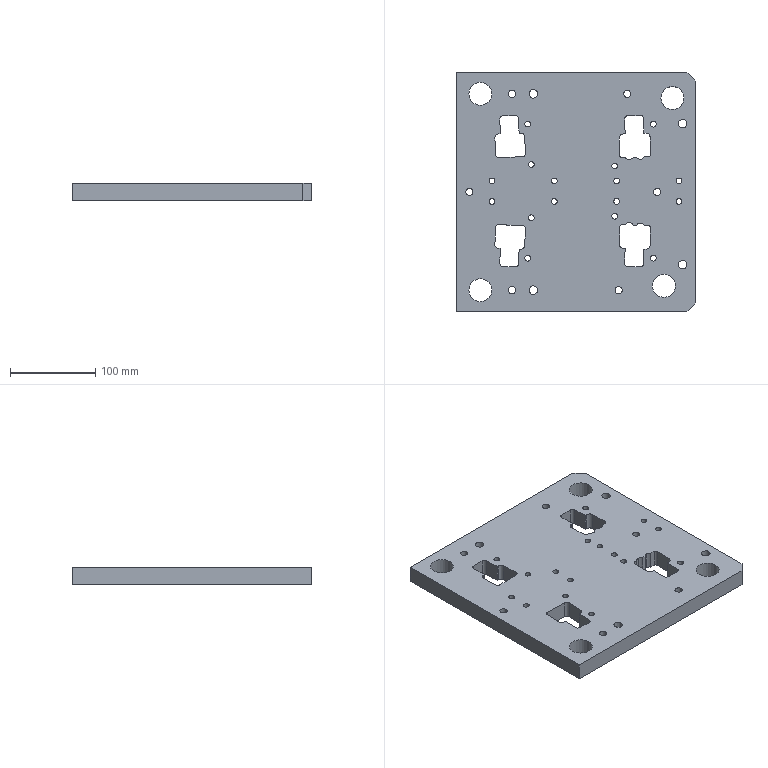Part | NX | features PPS-3 2 | 1 solid | 126 faces | box 280 x 280 x 20 mm | volume 1379962 mm3 | cylinder 60 | plane 44 | cone 14 | spline 8 | commonest cylinder face diameters 7 x12 10 x10 6.8 x8 6.805 x8 9 x8 8.5 x6